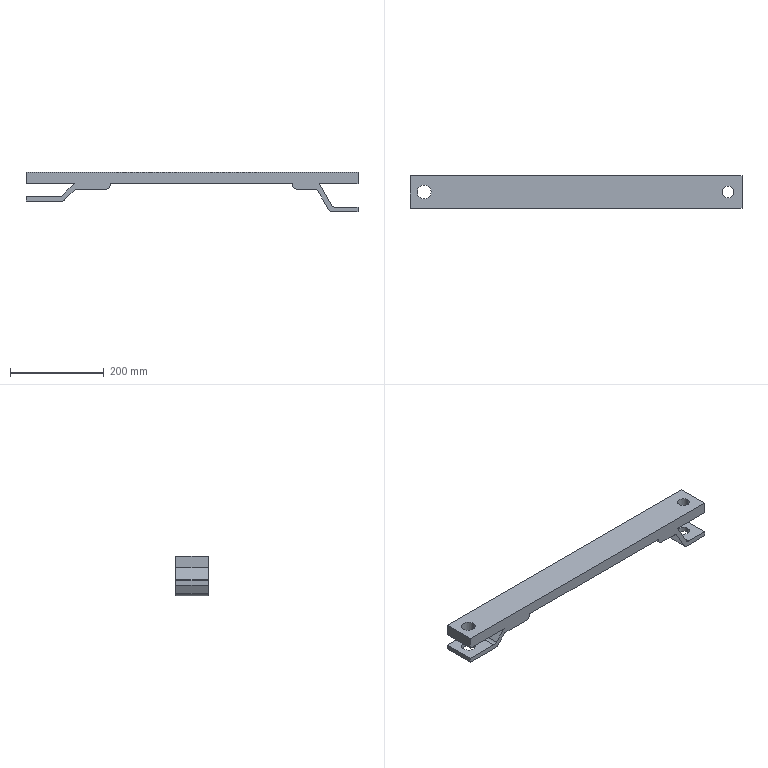Part | SolidWorks | 1 solid | 37 faces | box 710 x 70 x 85 mm | volume 1467586 mm3 | plane 22 | cylinder 15 | commonest cylinder face diameters 20 x7 25 x4 30 x4
STEP:
#1=CARTESIAN_POINT('',(692.5,35.,0.));
#2=VERTEX_POINT('',#1);
#3=CARTESIAN_POINT('',(667.5,35.,0.));
#4=VERTEX_POINT('',#3);
#5=CARTESIAN_POINT('',(680.,35.,0.));
#6=DIRECTION('',(0.,0.,-1.));
#7=DIRECTION('',(-1.,0.,0.));
#8=AXIS2_PLACEMENT_3D('',#5,#6,#7);
#9=CIRCLE('',#8,12.5);
#10=EDGE_CURVE('',#2,#4,#9,.T.);
#11=ORIENTED_EDGE('',*,*,#10,.F.);
#12=CARTESIAN_POINT('',(692.5,35.,-25.));
#13=VERTEX_POINT('',#12);
#14=CARTESIAN_POINT('',(692.5,35.,39.));
#15=DIRECTION('',(0.,0.,-1.));
#16=VECTOR('',#15,1000.);
#17=LINE('',#14,#16);
#18=EDGE_CURVE('',#2,#13,#17,.T.);
#19=ORIENTED_EDGE('',*,*,#18,.T.);
#20=CARTESIAN_POINT('',(667.5,35.,-25.));
#21=VERTEX_POINT('',#20);
#22=CARTESIAN_POINT('',(680.,35.,-25.));
#23=DIRECTION('',(0.,0.,-1.));
#24=DIRECTION('',(-1.,0.,0.));
#25=AXIS2_PLACEMENT_3D('',#22,#23,#24);
#26=CIRCLE('',#25,12.5);
#27=EDGE_CURVE('',#13,#21,#26,.T.);
#28=ORIENTED_EDGE('',*,*,#27,.T.);
#29=CARTESIAN_POINT('',(667.5,35.,39.));
#30=DIRECTION('',(0.,0.,-1.));
#31=VECTOR('',#30,1000.);
#32=LINE('',#29,#31);
#33=EDGE_CURVE('',#4,#21,#32,.T.);
#34=ORIENTED_EDGE('',*,*,#33,.F.);
#35=EDGE_LOOP('',(#11,#19,#28,#34));
#36=FACE_OUTER_BOUND('',#35,.T.);
#37=CARTESIAN_POINT('',(680.,35.,39.));
#38=DIRECTION('',(0.,0.,-1.));
#39=DIRECTION('',(-1.,0.,0.));
#40=AXIS2_PLACEMENT_3D('',#37,#38,#39);
#41=CYLINDRICAL_SURFACE('',#40,12.5);
#42=ADVANCED_FACE('',(#36),#41,.F.);
#43=CARTESIAN_POINT('',(692.5,35.,-75.));
#44=VERTEX_POINT('',#43);
#45=CARTESIAN_POINT('',(667.5,35.,-75.));
#46=VERTEX_POINT('',#45);
#47=CARTESIAN_POINT('',(680.,35.,-75.));
#48=DIRECTION('',(0.,0.,-1.));
#49=DIRECTION('',(-1.,0.,0.));
#50=AXIS2_PLACEMENT_3D('',#47,#48,#49);
#51=CIRCLE('',#50,12.5);
#52=EDGE_CURVE('',#44,#46,#51,.T.);
#53=ORIENTED_EDGE('',*,*,#52,.F.);
#54=CARTESIAN_POINT('',(692.5,35.,-85.));
#55=VERTEX_POINT('',#54);
#56=CARTESIAN_POINT('',(692.5,35.,39.));
#57=DIRECTION('',(0.,0.,-1.));
#58=VECTOR('',#57,1000.);
#59=LINE('',#56,#58);
#60=EDGE_CURVE('',#44,#55,#59,.T.);
#61=ORIENTED_EDGE('',*,*,#60,.T.);
#62=CARTESIAN_POINT('',(667.5,35.,-85.));
#63=VERTEX_POINT('',#62);
#64=CARTESIAN_POINT('',(680.,35.,-85.));
#65=DIRECTION('',(0.,0.,-1.));
#66=DIRECTION('',(-1.,0.,0.));
#67=AXIS2_PLACEMENT_3D('',#64,#65,#66);
#68=CIRCLE('',#67,12.5);
#69=EDGE_CURVE('',#55,#63,#68,.T.);
#70=ORIENTED_EDGE('',*,*,#69,.T.);
#71=CARTESIAN_POINT('',(667.5,35.,39.));
#72=DIRECTION('',(0.,0.,-1.));
#73=VECTOR('',#72,1000.);
#74=LINE('',#71,#73);
#75=EDGE_CURVE('',#46,#63,#74,.T.);
#76=ORIENTED_EDGE('',*,*,#75,.F.);
#77=EDGE_LOOP('',(#53,#61,#70,#76));
#78=FACE_OUTER_BOUND('',#77,.T.);
#79=CARTESIAN_POINT('',(680.,35.,39.));
#80=DIRECTION('',(0.,0.,-1.));
#81=DIRECTION('',(-1.,0.,0.));
#82=AXIS2_PLACEMENT_3D('',#79,#80,#81);
#83=CYLINDRICAL_SURFACE('',#82,12.5);
#84=ADVANCED_FACE('',(#78),#83,.F.);
#85=CARTESIAN_POINT('',(45.,35.,-52.));
#86=VERTEX_POINT('',#85);
#87=CARTESIAN_POINT('',(15.,35.,-52.));
#88=VERTEX_POINT('',#87);
#89=CARTESIAN_POINT('',(30.,35.,-52.));
#90=DIRECTION('',(0.,0.,-1.));
#91=DIRECTION('',(-1.,0.,0.));
#92=AXIS2_PLACEMENT_3D('',#89,#90,#91);
#93=CIRCLE('',#92,15.);
#94=EDGE_CURVE('',#86,#88,#93,.T.);
#95=ORIENTED_EDGE('',*,*,#94,.F.);
#96=CARTESIAN_POINT('',(45.,35.,-62.));
#97=VERTEX_POINT('',#96);
#98=CARTESIAN_POINT('',(45.,35.,39.));
#99=DIRECTION('',(0.,0.,-1.));
#100=VECTOR('',#99,1000.);
#101=LINE('',#98,#100);
#102=EDGE_CURVE('',#86,#97,#101,.T.);
#103=ORIENTED_EDGE('',*,*,#102,.T.);
#104=CARTESIAN_POINT('',(15.,35.,-62.));
#105=VERTEX_POINT('',#104);
#106=CARTESIAN_POINT('',(30.,35.,-62.));
#107=DIRECTION('',(0.,0.,-1.));
#108=DIRECTION('',(-1.,0.,0.));
#109=AXIS2_PLACEMENT_3D('',#106,#107,#108);
#110=CIRCLE('',#109,15.);
#111=EDGE_CURVE('',#97,#105,#110,.T.);
#112=ORIENTED_EDGE('',*,*,#111,.T.);
#113=CARTESIAN_POINT('',(15.,35.,39.));
#114=DIRECTION('',(0.,0.,-1.));
#115=VECTOR('',#114,1000.);
#116=LINE('',#113,#115);
#117=EDGE_CURVE('',#88,#105,#116,.T.);
#118=ORIENTED_EDGE('',*,*,#117,.F.);
#119=EDGE_LOOP('',(#95,#103,#112,#118));
#120=FACE_OUTER_BOUND('',#119,.T.);
#121=CARTESIAN_POINT('',(30.,35.,39.));
#122=DIRECTION('',(0.,0.,-1.));
#123=DIRECTION('',(-1.,0.,0.));
#124=AXIS2_PLACEMENT_3D('',#121,#122,#123);
#125=CYLINDRICAL_SURFACE('',#124,15.);
#126=ADVANCED_FACE('',(#120),#125,.F.);
#127=CARTESIAN_POINT('',(45.,35.,0.));
#128=VERTEX_POINT('',#127);
#129=CARTESIAN_POINT('',(15.,35.,0.));
#130=VERTEX_POINT('',#129);
#131=CARTESIAN_POINT('',(30.,35.,0.));
#132=DIRECTION('',(0.,0.,-1.));
#133=DIRECTION('',(-1.,0.,0.));
#134=AXIS2_PLACEMENT_3D('',#131,#132,#133);
#135=CIRCLE('',#134,15.);
#136=EDGE_CURVE('',#128,#130,#135,.T.);
#137=ORIENTED_EDGE('',*,*,#136,.F.);
#138=CARTESIAN_POINT('',(45.,35.,-25.));
#139=VERTEX_POINT('',#138);
#140=CARTESIAN_POINT('',(45.,35.,39.));
#141=DIRECTION('',(0.,0.,-1.));
#142=VECTOR('',#141,1000.);
#143=LINE('',#140,#142);
#144=EDGE_CURVE('',#128,#139,#143,.T.);
#145=ORIENTED_EDGE('',*,*,#144,.T.);
#146=CARTESIAN_POINT('',(15.,35.,-25.));
#147=VERTEX_POINT('',#146);
#148=CARTESIAN_POINT('',(30.,35.,-25.));
#149=DIRECTION('',(0.,0.,-1.));
#150=DIRECTION('',(-1.,0.,0.));
#151=AXIS2_PLACEMENT_3D('',#148,#149,#150);
#152=CIRCLE('',#151,15.);
#153=EDGE_CURVE('',#139,#147,#152,.T.);
#154=ORIENTED_EDGE('',*,*,#153,.T.);
#155=CARTESIAN_POINT('',(15.,35.,39.));
#156=DIRECTION('',(0.,0.,-1.));
#157=VECTOR('',#156,1000.);
#158=LINE('',#155,#157);
#159=EDGE_CURVE('',#130,#147,#158,.T.);
#160=ORIENTED_EDGE('',*,*,#159,.F.);
#161=EDGE_LOOP('',(#137,#145,#154,#160));
#162=FACE_OUTER_BOUND('',#161,.T.);
#163=CARTESIAN_POINT('',(30.,35.,39.));
#164=DIRECTION('',(0.,0.,-1.));
#165=DIRECTION('',(-1.,0.,0.));
#166=AXIS2_PLACEMENT_3D('',#163,#164,#165);
#167=CYLINDRICAL_SURFACE('',#166,15.);
#168=ADVANCED_FACE('',(#162),#167,.F.);
#169=CARTESIAN_POINT('',(680.,35.,0.));
#170=DIRECTION('',(0.,0.,-1.));
#171=DIRECTION('',(-1.,0.,0.));
#172=AXIS2_PLACEMENT_3D('',#169,#170,#171);
#173=CIRCLE('',#172,12.5);
#174=EDGE_CURVE('',#4,#2,#173,.T.);
#175=ORIENTED_EDGE('',*,*,#174,.T.);
#176=ORIENTED_EDGE('',*,*,#10,.T.);
#177=EDGE_LOOP('',(#175,#176));
#178=FACE_BOUND('',#177,.T.);
#179=CARTESIAN_POINT('',(30.,35.,0.));
#180=DIRECTION('',(0.,0.,-1.));
#181=DIRECTION('',(-1.,0.,0.));
#182=AXIS2_PLACEMENT_3D('',#179,#180,#181);
#183=CIRCLE('',#182,15.);
#184=EDGE_CURVE('',#130,#128,#183,.T.);
#185=ORIENTED_EDGE('',*,*,#184,.T.);
#186=ORIENTED_EDGE('',*,*,#136,.T.);
#187=EDGE_LOOP('',(#185,#186));
#188=FACE_BOUND('',#187,.T.);
#189=CARTESIAN_POINT('',(0.,0.,0.));
#190=VERTEX_POINT('',#189);
#191=CARTESIAN_POINT('',(710.,0.,0.));
#192=VERTEX_POINT('',#191);
#193=CARTESIAN_POINT('',(0.,0.,0.));
#194=DIRECTION('',(1.,0.,0.));
#195=VECTOR('',#194,1000.);
#196=LINE('',#193,#195);
#197=EDGE_CURVE('',#190,#192,#196,.T.);
#198=ORIENTED_EDGE('',*,*,#197,.T.);
#199=CARTESIAN_POINT('',(710.,70.,0.));
#200=VERTEX_POINT('',#199);
#201=CARTESIAN_POINT('',(710.,70.,0.));
#202=DIRECTION('',(0.,-1.,0.));
#203=VECTOR('',#202,1000.);
#204=LINE('',#201,#203);
#205=EDGE_CURVE('',#200,#192,#204,.T.);
#206=ORIENTED_EDGE('',*,*,#205,.F.);
#207=CARTESIAN_POINT('',(0.,70.,0.));
#208=VERTEX_POINT('',#207);
#209=CARTESIAN_POINT('',(0.,70.,0.));
#210=DIRECTION('',(1.,0.,0.));
#211=VECTOR('',#210,1000.);
#212=LINE('',#209,#211);
#213=EDGE_CURVE('',#208,#200,#212,.T.);
#214=ORIENTED_EDGE('',*,*,#213,.F.);
#215=CARTESIAN_POINT('',(0.,70.,0.));
#216=DIRECTION('',(0.,-1.,0.));
#217=VECTOR('',#216,1000.);
#218=LINE('',#215,#217);
#219=EDGE_CURVE('',#208,#190,#218,.T.);
#220=ORIENTED_EDGE('',*,*,#219,.T.);
#221=EDGE_LOOP('',(#198,#206,#214,#220));
#222=FACE_OUTER_BOUND('',#221,.T.);
#223=CARTESIAN_POINT('',(0.,70.,0.));
#224=DIRECTION('',(0.,0.,-1.));
#225=DIRECTION('',(-1.,0.,0.));
#226=AXIS2_PLACEMENT_3D('',#223,#224,#225);
#227=PLANE('',#226);
#228=ADVANCED_FACE('',(#178,#188,#222),#227,.F.);
#229=CARTESIAN_POINT('',(710.,0.,-25.));
#230=VERTEX_POINT('',#229);
#231=CARTESIAN_POINT('',(710.,0.,0.));
#232=DIRECTION('',(0.,0.,-1.));
#233=VECTOR('',#232,1000.);
#234=LINE('',#231,#233);
#235=EDGE_CURVE('',#192,#230,#234,.T.);
#236=ORIENTED_EDGE('',*,*,#235,.T.);
#237=CARTESIAN_POINT('',(710.,70.,-25.));
#238=VERTEX_POINT('',#237);
#239=CARTESIAN_POINT('',(710.,70.,-25.));
#240=DIRECTION('',(0.,-1.,0.));
#241=VECTOR('',#240,1000.);
#242=LINE('',#239,#241);
#243=EDGE_CURVE('',#238,#230,#242,.T.);
#244=ORIENTED_EDGE('',*,*,#243,.F.);
#245=CARTESIAN_POINT('',(710.,70.,0.));
#246=DIRECTION('',(0.,0.,-1.));
#247=VECTOR('',#246,1000.);
#248=LINE('',#245,#247);
#249=EDGE_CURVE('',#200,#238,#248,.T.);
#250=ORIENTED_EDGE('',*,*,#249,.F.);
#251=ORIENTED_EDGE('',*,*,#205,.T.);
#252=EDGE_LOOP('',(#236,#244,#250,#251));
#253=FACE_OUTER_BOUND('',#252,.T.);
#254=CARTESIAN_POINT('',(710.,70.,0.));
#255=DIRECTION('',(-1.,0.,0.));
#256=DIRECTION('',(0.,0.,1.));
#257=AXIS2_PLACEMENT_3D('',#254,#255,#256);
#258=PLANE('',#257);
#259=ADVANCED_FACE('',(#253),#258,.F.);
#260=CARTESIAN_POINT('',(680.,35.,-25.));
#261=DIRECTION('',(0.,0.,-1.));
#262=DIRECTION('',(-1.,0.,0.));
#263=AXIS2_PLACEMENT_3D('',#260,#261,#262);
#264=CIRCLE('',#263,12.5);
#265=EDGE_CURVE('',#21,#13,#264,.T.);
#266=ORIENTED_EDGE('',*,*,#265,.F.);
#267=ORIENTED_EDGE('',*,*,#27,.F.);
#268=EDGE_LOOP('',(#266,#267));
#269=FACE_BOUND('',#268,.T.);
#270=CARTESIAN_POINT('',(626.906,0.,-25.));
#271=VERTEX_POINT('',#270);
#272=CARTESIAN_POINT('',(0.,0.,-25.));
#273=DIRECTION('',(1.,0.,0.));
#274=VECTOR('',#273,1000.);
#275=LINE('',#272,#274);
#276=EDGE_CURVE('',#271,#230,#275,.T.);
#277=ORIENTED_EDGE('',*,*,#276,.F.);
#278=CARTESIAN_POINT('',(626.906,70.,-25.));
#279=VERTEX_POINT('',#278);
#280=CARTESIAN_POINT('',(626.906,70.,-25.));
#281=DIRECTION('',(0.,-1.,0.));
#282=VECTOR('',#281,1000.);
#283=LINE('',#280,#282);
#284=EDGE_CURVE('',#279,#271,#283,.T.);
#285=ORIENTED_EDGE('',*,*,#284,.F.);
#286=CARTESIAN_POINT('',(0.,70.,-25.));
#287=DIRECTION('',(1.,0.,0.));
#288=VECTOR('',#287,1000.);
#289=LINE('',#286,#288);
#290=EDGE_CURVE('',#279,#238,#289,.T.);
#291=ORIENTED_EDGE('',*,*,#290,.T.);
#292=ORIENTED_EDGE('',*,*,#243,.T.);
#293=EDGE_LOOP('',(#277,#285,#291,#292));
#294=FACE_OUTER_BOUND('',#293,.T.);
#295=CARTESIAN_POINT('',(0.,70.,-25.));
#296=DIRECTION('',(0.,0.,-1.));
#297=DIRECTION('',(-1.,0.,0.));
#298=AXIS2_PLACEMENT_3D('',#295,#296,#297);
#299=PLANE('',#298);
#300=ADVANCED_FACE('',(#269,#294),#299,.T.);
#301=CARTESIAN_POINT('',(652.887,0.,-70.));
#302=VERTEX_POINT('',#301);
#303=CARTESIAN_POINT('',(459.354,0.,265.208));
#304=DIRECTION('',(0.5,0.,-0.866));
#305=VECTOR('',#304,1000.);
#306=LINE('',#303,#305);
#307=EDGE_CURVE('',#271,#302,#306,.T.);
#308=ORIENTED_EDGE('',*,*,#307,.T.);
#309=CARTESIAN_POINT('',(652.887,70.,-70.));
#310=VERTEX_POINT('',#309);
#311=CARTESIAN_POINT('',(652.887,70.,-70.));
#312=DIRECTION('',(0.,1.,0.));
#313=VECTOR('',#312,1000.);
#314=LINE('',#311,#313);
#315=EDGE_CURVE('',#302,#310,#314,.T.);
#316=ORIENTED_EDGE('',*,*,#315,.T.);
#317=CARTESIAN_POINT('',(459.354,70.,265.208));
#318=DIRECTION('',(0.5,0.,-0.866));
#319=VECTOR('',#318,1000.);
#320=LINE('',#317,#319);
#321=EDGE_CURVE('',#279,#310,#320,.T.);
#322=ORIENTED_EDGE('',*,*,#321,.F.);
#323=ORIENTED_EDGE('',*,*,#284,.T.);
#324=EDGE_LOOP('',(#308,#316,#322,#323));
#325=FACE_OUTER_BOUND('',#324,.T.);
#326=CARTESIAN_POINT('',(459.354,70.,265.208));
#327=DIRECTION('',(-0.866,0.,-0.5));
#328=DIRECTION('',(-0.5,0.,0.866));
#329=AXIS2_PLACEMENT_3D('',#326,#327,#328);
#330=PLANE('',#329);
#331=ADVANCED_FACE('',(#325),#330,.F.);
#332=CARTESIAN_POINT('',(680.,35.,-75.));
#333=DIRECTION('',(0.,0.,-1.));
#334=DIRECTION('',(-1.,0.,0.));
#335=AXIS2_PLACEMENT_3D('',#332,#333,#334);
#336=CIRCLE('',#335,12.5);
#337=EDGE_CURVE('',#46,#44,#336,.T.);
#338=ORIENTED_EDGE('',*,*,#337,.T.);
#339=ORIENTED_EDGE('',*,*,#52,.T.);
#340=EDGE_LOOP('',(#338,#339));
#341=FACE_BOUND('',#340,.T.);
#342=CARTESIAN_POINT('',(661.547,70.,-75.));
#343=VERTEX_POINT('',#342);
#344=CARTESIAN_POINT('',(710.,70.,-75.));
#345=VERTEX_POINT('',#344);
#346=CARTESIAN_POINT('',(0.,70.,-75.));
#347=DIRECTION('',(1.,0.,0.));
#348=VECTOR('',#347,1000.);
#349=LINE('',#346,#348);
#350=EDGE_CURVE('',#343,#345,#349,.T.);
#351=ORIENTED_EDGE('',*,*,#350,.F.);
#352=CARTESIAN_POINT('',(661.547,0.,-75.));
#353=VERTEX_POINT('',#352);
#354=CARTESIAN_POINT('',(661.547,0.,-75.));
#355=DIRECTION('',(0.,-1.,0.));
#356=VECTOR('',#355,1000.);
#357=LINE('',#354,#356);
#358=EDGE_CURVE('',#343,#353,#357,.T.);
#359=ORIENTED_EDGE('',*,*,#358,.T.);
#360=CARTESIAN_POINT('',(710.,0.,-75.));
#361=VERTEX_POINT('',#360);
#362=CARTESIAN_POINT('',(0.,0.,-75.));
#363=DIRECTION('',(1.,0.,0.));
#364=VECTOR('',#363,1000.);
#365=LINE('',#362,#364);
#366=EDGE_CURVE('',#353,#361,#365,.T.);
#367=ORIENTED_EDGE('',*,*,#366,.T.);
#368=CARTESIAN_POINT('',(710.,70.,-75.));
#369=DIRECTION('',(0.,-1.,0.));
#370=VECTOR('',#369,1000.);
#371=LINE('',#368,#370);
#372=EDGE_CURVE('',#345,#361,#371,.T.);
#373=ORIENTED_EDGE('',*,*,#372,.F.);
#374=EDGE_LOOP('',(#351,#359,#367,#373));
#375=FACE_OUTER_BOUND('',#374,.T.);
#376=CARTESIAN_POINT('',(0.,70.,-75.));
#377=DIRECTION('',(0.,0.,-1.));
#378=DIRECTION('',(-1.,0.,0.));
#379=AXIS2_PLACEMENT_3D('',#376,#377,#378);
#380=PLANE('',#379);
#381=ADVANCED_FACE('',(#341,#375),#380,.F.);
#382=CARTESIAN_POINT('',(710.,0.,-85.));
#383=VERTEX_POINT('',#382);
#384=CARTESIAN_POINT('',(710.,0.,0.));
#385=DIRECTION('',(0.,0.,1.));
#386=VECTOR('',#385,1000.);
#387=LINE('',#384,#386);
#388=EDGE_CURVE('',#383,#361,#387,.T.);
#389=ORIENTED_EDGE('',*,*,#388,.F.);
#390=CARTESIAN_POINT('',(710.,70.,-85.));
#391=VERTEX_POINT('',#390);
#392=CARTESIAN_POINT('',(710.,70.,-85.));
#393=DIRECTION('',(0.,-1.,0.));
#394=VECTOR('',#393,1000.);
#395=LINE('',#392,#394);
#396=EDGE_CURVE('',#391,#383,#395,.T.);
#397=ORIENTED_EDGE('',*,*,#396,.F.);
#398=CARTESIAN_POINT('',(710.,70.,0.));
#399=DIRECTION('',(0.,0.,1.));
#400=VECTOR('',#399,1000.);
#401=LINE('',#398,#400);
#402=EDGE_CURVE('',#391,#345,#401,.T.);
#403=ORIENTED_EDGE('',*,*,#402,.T.);
#404=ORIENTED_EDGE('',*,*,#372,.T.);
#405=EDGE_LOOP('',(#389,#397,#403,#404));
#406=FACE_OUTER_BOUND('',#405,.T.);
#407=CARTESIAN_POINT('',(710.,70.,0.));
#408=DIRECTION('',(1.,0.,0.));
#409=DIRECTION('',(0.,0.,-1.));
#410=AXIS2_PLACEMENT_3D('',#407,#408,#409);
#411=PLANE('',#410);
#412=ADVANCED_FACE('',(#406),#411,.T.);
#413=CARTESIAN_POINT('',(680.,35.,-85.));
#414=DIRECTION('',(0.,0.,-1.));
#415=DIRECTION('',(-1.,0.,0.));
#416=AXIS2_PLACEMENT_3D('',#413,#414,#415);
#417=CIRCLE('',#416,12.5);
#418=EDGE_CURVE('',#63,#55,#417,.T.);
#419=ORIENTED_EDGE('',*,*,#418,.F.);
#420=ORIENTED_EDGE('',*,*,#69,.F.);
#421=EDGE_LOOP('',(#419,#420));
#422=FACE_BOUND('',#421,.T.);
#423=CARTESIAN_POINT('',(655.774,0.,-85.));
#424=VERTEX_POINT('',#423);
#425=CARTESIAN_POINT('',(0.,0.,-85.));
#426=DIRECTION('',(1.,0.,0.));
#427=VECTOR('',#426,1000.);
#428=LINE('',#425,#427);
#429=EDGE_CURVE('',#424,#383,#428,.T.);
#430=ORIENTED_EDGE('',*,*,#429,.F.);
#431=CARTESIAN_POINT('',(655.774,70.,-85.));
#432=VERTEX_POINT('',#431);
#433=CARTESIAN_POINT('',(655.774,70.,-85.));
#434=DIRECTION('',(0.,1.,0.));
#435=VECTOR('',#434,1000.);
#436=LINE('',#433,#435);
#437=EDGE_CURVE('',#424,#432,#436,.T.);
#438=ORIENTED_EDGE('',*,*,#437,.T.);
#439=CARTESIAN_POINT('',(0.,70.,-85.));
#440=DIRECTION('',(1.,0.,0.));
#441=VECTOR('',#440,1000.);
#442=LINE('',#439,#441);
#443=EDGE_CURVE('',#432,#391,#442,.T.);
#444=ORIENTED_EDGE('',*,*,#443,.T.);
#445=ORIENTED_EDGE('',*,*,#396,.T.);
#446=EDGE_LOOP('',(#430,#438,#444,#445));
#447=FACE_OUTER_BOUND('',#446,.T.);
#448=CARTESIAN_POINT('',(0.,70.,-85.));
#449=DIRECTION('',(0.,0.,-1.));
#450=DIRECTION('',(-1.,0.,0.));
#451=AXIS2_PLACEMENT_3D('',#448,#449,#450);
#452=PLANE('',#451);
#453=ADVANCED_FACE('',(#422,#447),#452,.T.);
#454=CARTESIAN_POINT('',(625.174,0.,-42.));
#455=VERTEX_POINT('',#454);
#456=CARTESIAN_POINT('',(647.113,0.,-80.));
#457=VERTEX_POINT('',#456);
#458=CARTESIAN_POINT('',(450.694,0.,260.208));
#459=DIRECTION('',(0.5,0.,-0.866));
#460=VECTOR('',#459,1000.);
#461=LINE('',#458,#460);
#462=EDGE_CURVE('',#455,#457,#461,.T.);
#463=ORIENTED_EDGE('',*,*,#462,.F.);
#464=CARTESIAN_POINT('',(625.174,70.,-42.));
#465=VERTEX_POINT('',#464);
#466=CARTESIAN_POINT('',(625.174,70.,-42.));
#467=DIRECTION('',(0.,1.,0.));
#468=VECTOR('',#467,1000.);
#469=LINE('',#466,#468);
#470=EDGE_CURVE('',#455,#465,#469,.T.);
#471=ORIENTED_EDGE('',*,*,#470,.T.);
#472=CARTESIAN_POINT('',(647.113,70.,-80.));
#473=VERTEX_POINT('',#472);
#474=CARTESIAN_POINT('',(450.694,70.,260.208));
#475=DIRECTION('',(0.5,0.,-0.866));
#476=VECTOR('',#475,1000.);
#477=LINE('',#474,#476);
#478=EDGE_CURVE('',#465,#473,#477,.T.);
#479=ORIENTED_EDGE('',*,*,#478,.T.);
#480=CARTESIAN_POINT('',(647.113,70.,-80.));
#481=DIRECTION('',(0.,-1.,0.));
#482=VECTOR('',#481,1000.);
#483=LINE('',#480,#482);
#484=EDGE_CURVE('',#473,#457,#483,.T.);
#485=ORIENTED_EDGE('',*,*,#484,.T.);
#486=EDGE_LOOP('',(#463,#471,#479,#485));
#487=FACE_OUTER_BOUND('',#486,.T.);
#488=CARTESIAN_POINT('',(450.694,70.,260.208));
#489=DIRECTION('',(-0.866,0.,-0.5));
#490=DIRECTION('',(-0.5,0.,0.866));
#491=AXIS2_PLACEMENT_3D('',#488,#489,#490);
#492=PLANE('',#491);
#493=ADVANCED_FACE('',(#487),#492,.T.);
#494=CARTESIAN_POINT('',(580.,0.,-37.));
#495=VERTEX_POINT('',#494);
#496=CARTESIAN_POINT('',(616.514,0.,-37.));
#497=VERTEX_POINT('',#496);
#498=CARTESIAN_POINT('',(0.,0.,-37.));
#499=DIRECTION('',(1.,0.,0.));
#500=VECTOR('',#499,1000.);
#501=LINE('',#498,#500);
#502=EDGE_CURVE('',#495,#497,#501,.T.);
#503=ORIENTED_EDGE('',*,*,#502,.F.);
#504=CARTESIAN_POINT('',(580.,70.,-37.));
#505=VERTEX_POINT('',#504);
#506=CARTESIAN_POINT('',(580.,70.,-37.));
#507=DIRECTION('',(0.,1.,0.));
#508=VECTOR('',#507,1000.);
#509=LINE('',#506,#508);
#510=EDGE_CURVE('',#495,#505,#509,.T.);
#511=ORIENTED_EDGE('',*,*,#510,.T.);
#512=CARTESIAN_POINT('',(616.514,70.,-37.));
#513=VERTEX_POINT('',#512);
#514=CARTESIAN_POINT('',(0.,70.,-37.));
#515=DIRECTION('',(1.,0.,0.));
#516=VECTOR('',#515,1000.);
#517=LINE('',#514,#516);
#518=EDGE_CURVE('',#505,#513,#517,.T.);
#519=ORIENTED_EDGE('',*,*,#518,.T.);
#520=CARTESIAN_POINT('',(616.514,0.,-37.));
#521=DIRECTION('',(0.,-1.,0.));
#522=VECTOR('',#521,1000.);
#523=LINE('',#520,#522);
#524=EDGE_CURVE('',#513,#497,#523,.T.);
#525=ORIENTED_EDGE('',*,*,#524,.T.);
#526=EDGE_LOOP('',(#503,#511,#519,#525));
#527=FACE_OUTER_BOUND('',#526,.T.);
#528=CARTESIAN_POINT('',(0.,70.,-37.));
#529=DIRECTION('',(0.,0.,-1.));
#530=DIRECTION('',(-1.,0.,0.));
#531=AXIS2_PLACEMENT_3D('',#528,#529,#530);
#532=PLANE('',#531);
#533=ADVANCED_FACE('',(#527),#532,.T.);
#534=CARTESIAN_POINT('',(570.,70.,-25.));
#535=VERTEX_POINT('',#534);
#536=CARTESIAN_POINT('',(570.,70.,-27.));
#537=VERTEX_POINT('',#536);
#538=CARTESIAN_POINT('',(570.,70.,0.));
#539=DIRECTION('',(0.,0.,-1.));
#540=VECTOR('',#539,1000.);
#541=LINE('',#538,#540);
#542=EDGE_CURVE('',#535,#537,#541,.T.);
#543=ORIENTED_EDGE('',*,*,#542,.T.);
#544=CARTESIAN_POINT('',(570.,0.,-27.));
#545=VERTEX_POINT('',#544);
#546=CARTESIAN_POINT('',(570.,70.,-27.));
#547=DIRECTION('',(0.,-1.,0.));
#548=VECTOR('',#547,1000.);
#549=LINE('',#546,#548);
#550=EDGE_CURVE('',#537,#545,#549,.T.);
#551=ORIENTED_EDGE('',*,*,#550,.T.);
#552=CARTESIAN_POINT('',(570.,0.,-25.));
#553=VERTEX_POINT('',#552);
#554=CARTESIAN_POINT('',(570.,0.,0.));
#555=DIRECTION('',(0.,0.,-1.));
#556=VECTOR('',#555,1000.);
#557=LINE('',#554,#556);
#558=EDGE_CURVE('',#553,#545,#557,.T.);
#559=ORIENTED_EDGE('',*,*,#558,.F.);
#560=CARTESIAN_POINT('',(570.,70.,-25.));
#561=DIRECTION('',(0.,-1.,0.));
#562=VECTOR('',#561,1000.);
#563=LINE('',#560,#562);
#564=EDGE_CURVE('',#535,#553,#563,.T.);
#565=ORIENTED_EDGE('',*,*,#564,.F.);
#566=EDGE_LOOP('',(#543,#551,#559,#565));
#567=FACE_OUTER_BOUND('',#566,.T.);
#568=CARTESIAN_POINT('',(570.,70.,0.));
#569=DIRECTION('',(-1.,0.,0.));
#570=DIRECTION('',(0.,0.,1.));
#571=AXIS2_PLACEMENT_3D('',#568,#569,#570);
#572=PLANE('',#571);
#573=ADVANCED_FACE('',(#567),#572,.T.);
#574=CARTESIAN_POINT('',(180.,0.,-25.));
#575=VERTEX_POINT('',#574);
#576=CARTESIAN_POINT('',(0.,0.,-25.));
#577=DIRECTION('',(1.,0.,0.));
#578=VECTOR('',#577,1000.);
#579=LINE('',#576,#578);
#580=EDGE_CURVE('',#575,#553,#579,.T.);
#581=ORIENTED_EDGE('',*,*,#580,.F.);
#582=CARTESIAN_POINT('',(180.,70.,-25.));
#583=VERTEX_POINT('',#582);
#584=CARTESIAN_POINT('',(180.,70.,-25.));
#585=DIRECTION('',(0.,-1.,0.));
#586=VECTOR('',#585,1000.);
#587=LINE('',#584,#586);
#588=EDGE_CURVE('',#583,#575,#587,.T.);
#589=ORIENTED_EDGE('',*,*,#588,.F.);
#590=CARTESIAN_POINT('',(0.,70.,-25.));
#591=DIRECTION('',(1.,0.,0.));
#592=VECTOR('',#591,1000.);
#593=LINE('',#590,#592);
#594=EDGE_CURVE('',#583,#535,#593,.T.);
#595=ORIENTED_EDGE('',*,*,#594,.T.);
#596=ORIENTED_EDGE('',*,*,#564,.T.);
#597=EDGE_LOOP('',(#581,#589,#595,#596));
#598=FACE_OUTER_BOUND('',#597,.T.);
#599=CARTESIAN_POINT('',(0.,70.,-25.));
#600=DIRECTION('',(0.,0.,-1.));
#601=DIRECTION('',(-1.,0.,0.));
#602=AXIS2_PLACEMENT_3D('',#599,#600,#601);
#603=PLANE('',#602);
#604=ADVANCED_FACE('',(#598),#603,.T.);
#605=CARTESIAN_POINT('',(180.,0.,-27.));
#606=VERTEX_POINT('',#605);
#607=CARTESIAN_POINT('',(180.,0.,0.));
#608=DIRECTION('',(0.,0.,1.));
#609=VECTOR('',#608,1000.);
#610=LINE('',#607,#609);
#611=EDGE_CURVE('',#606,#575,#610,.T.);
#612=ORIENTED_EDGE('',*,*,#611,.F.);
#613=CARTESIAN_POINT('',(180.,70.,-27.));
#614=VERTEX_POINT('',#613);
#615=CARTESIAN_POINT('',(180.,70.,-27.));
#616=DIRECTION('',(0.,1.,0.));
#617=VECTOR('',#616,1000.);
#618=LINE('',#615,#617);
#619=EDGE_CURVE('',#606,#614,#618,.T.);
#620=ORIENTED_EDGE('',*,*,#619,.T.);
#621=CARTESIAN_POINT('',(180.,70.,0.));
#622=DIRECTION('',(0.,0.,1.));
#623=VECTOR('',#622,1000.);
#624=LINE('',#621,#623);
#625=EDGE_CURVE('',#614,#583,#624,.T.);
#626=ORIENTED_EDGE('',*,*,#625,.T.);
#627=ORIENTED_EDGE('',*,*,#588,.T.);
#628=EDGE_LOOP('',(#612,#620,#626,#627));
#629=FACE_OUTER_BOUND('',#628,.T.);
#630=CARTESIAN_POINT('',(180.,70.,0.));
#631=DIRECTION('',(1.,0.,0.));
#632=DIRECTION('',(0.,0.,-1.));
#633=AXIS2_PLACEMENT_3D('',#630,#631,#632);
#634=PLANE('',#633);
#635=ADVANCED_FACE('',(#629),#634,.T.);
#636=CARTESIAN_POINT('',(105.,70.,-37.));
#637=VERTEX_POINT('',#636);
#638=CARTESIAN_POINT('',(170.,70.,-37.));
#639=VERTEX_POINT('',#638);
#640=CARTESIAN_POINT('',(0.,70.,-37.));
#641=DIRECTION('',(1.,0.,0.));
#642=VECTOR('',#641,1000.);
#643=LINE('',#640,#642);
#644=EDGE_CURVE('',#637,#639,#643,.T.);
#645=ORIENTED_EDGE('',*,*,#644,.T.);
#646=CARTESIAN_POINT('',(170.,0.,-37.));
#647=VERTEX_POINT('',#646);
#648=CARTESIAN_POINT('',(170.,70.,-37.));
#649=DIRECTION('',(0.,-1.,0.));
#650=VECTOR('',#649,1000.);
#651=LINE('',#648,#650);
#652=EDGE_CURVE('',#639,#647,#651,.T.);
#653=ORIENTED_EDGE('',*,*,#652,.T.);
#654=CARTESIAN_POINT('',(105.,0.,-37.));
#655=VERTEX_POINT('',#654);
#656=CARTESIAN_POINT('',(0.,0.,-37.));
#657=DIRECTION('',(1.,0.,0.));
#658=VECTOR('',#657,1000.);
#659=LINE('',#656,#658);
#660=EDGE_CURVE('',#655,#647,#659,.T.);
#661=ORIENTED_EDGE('',*,*,#660,.F.);
#662=CARTESIAN_POINT('',(105.,70.,-37.));
#663=DIRECTION('',(0.,-1.,0.));
#664=VECTOR('',#663,1000.);
#665=LINE('',#662,#664);
#666=EDGE_CURVE('',#637,#655,#665,.T.);
#667=ORIENTED_EDGE('',*,*,#666,.F.);
#668=EDGE_LOOP('',(#645,#653,#661,#667));
#669=FACE_OUTER_BOUND('',#668,.T.);
#670=CARTESIAN_POINT('',(0.,70.,-37.));
#671=DIRECTION('',(0.,0.,-1.));
#672=DIRECTION('',(-1.,0.,0.));
#673=AXIS2_PLACEMENT_3D('',#670,#671,#672);
#674=PLANE('',#673);
#675=ADVANCED_FACE('',(#669),#674,.T.);
#676=CARTESIAN_POINT('',(82.929,0.,-59.071));
#677=VERTEX_POINT('',#676);
#678=CARTESIAN_POINT('',(71.,0.,-71.));
#679=DIRECTION('',(0.7071,0.,0.7071));
#680=VECTOR('',#679,1000.);
#681=LINE('',#678,#680);
#682=EDGE_CURVE('',#677,#655,#681,.T.);
#683=ORIENTED_EDGE('',*,*,#682,.F.);
#684=CARTESIAN_POINT('',(82.929,70.,-59.071));
#685=VERTEX_POINT('',#684);
#686=CARTESIAN_POINT('',(82.929,70.,-59.071));
#687=DIRECTION('',(0.,1.,0.));
#688=VECTOR('',#687,1000.);
#689=LINE('',#686,#688);
#690=EDGE_CURVE('',#677,#685,#689,.T.);
#691=ORIENTED_EDGE('',*,*,#690,.T.);
#692=CARTESIAN_POINT('',(71.,70.,-71.));
#693=DIRECTION('',(0.7071,0.,0.7071));
#694=VECTOR('',#693,1000.);
#695=LINE('',#692,#694);
#696=EDGE_CURVE('',#685,#637,#695,.T.);
#697=ORIENTED_EDGE('',*,*,#696,.T.);
#698=ORIENTED_EDGE('',*,*,#666,.T.);
#699=EDGE_LOOP('',(#683,#691,#697,#698));
#700=FACE_OUTER_BOUND('',#699,.T.);
#701=CARTESIAN_POINT('',(71.,70.,-71.));
#702=DIRECTION('',(0.7071,0.,-0.7071));
#703=DIRECTION('',(-0.7071,0.,-0.7071));
#704=AXIS2_PLACEMENT_3D('',#701,#702,#703);
#705=PLANE('',#704);
#706=ADVANCED_FACE('',(#700),#705,.T.);
#707=CARTESIAN_POINT('',(30.,35.,-62.));
#708=DIRECTION('',(0.,0.,-1.));
#709=DIRECTION('',(-1.,0.,0.));
#710=AXIS2_PLACEMENT_3D('',#707,#708,#709);
#711=CIRCLE('',#710,15.);
#712=EDGE_CURVE('',#105,#97,#711,.T.);
#713=ORIENTED_EDGE('',*,*,#712,.F.);
#714=ORIENTED_EDGE('',*,*,#111,.F.);
#715=EDGE_LOOP('',(#713,#714));
#716=FACE_BOUND('',#715,.T.);
#717=CARTESIAN_POINT('',(0.,70.,-62.));
#718=VERTEX_POINT('',#717);
#719=CARTESIAN_POINT('',(75.858,70.,-62.));
#720=VERTEX_POINT('',#719);
#721=CARTESIAN_POINT('',(0.,70.,-62.));
#722=DIRECTION('',(1.,0.,0.));
#723=VECTOR('',#722,1000.);
#724=LINE('',#721,#723);
#725=EDGE_CURVE('',#718,#720,#724,.T.);
#726=ORIENTED_EDGE('',*,*,#725,.T.);
#727=CARTESIAN_POINT('',(75.858,0.,-62.));
#728=VERTEX_POINT('',#727);
#729=CARTESIAN_POINT('',(75.858,70.,-62.));
#730=DIRECTION('',(0.,-1.,0.));
#731=VECTOR('',#730,1000.);
#732=LINE('',#729,#731);
#733=EDGE_CURVE('',#720,#728,#732,.T.);
#734=ORIENTED_EDGE('',*,*,#733,.T.);
#735=CARTESIAN_POINT('',(0.,0.,-62.));
#736=VERTEX_POINT('',#735);
#737=CARTESIAN_POINT('',(0.,0.,-62.));
#738=DIRECTION('',(1.,0.,0.));
#739=VECTOR('',#738,1000.);
#740=LINE('',#737,#739);
#741=EDGE_CURVE('',#736,#728,#740,.T.);
#742=ORIENTED_EDGE('',*,*,#741,.F.);
#743=CARTESIAN_POINT('',(0.,70.,-62.));
#744=DIRECTION('',(0.,-1.,0.));
#745=VECTOR('',#744,1000.);
#746=LINE('',#743,#745);
#747=EDGE_CURVE('',#718,#736,#746,.T.);
#748=ORIENTED_EDGE('',*,*,#747,.F.);
#749=EDGE_LOOP('',(#726,#734,#742,#748));
#750=FACE_OUTER_BOUND('',#749,.T.);
#751=CARTESIAN_POINT('',(0.,70.,-62.));
#752=DIRECTION('',(0.,0.,-1.));
#753=DIRECTION('',(-1.,0.,0.));
#754=AXIS2_PLACEMENT_3D('',#751,#752,#753);
#755=PLANE('',#754);
#756=ADVANCED_FACE('',(#716,#750),#755,.T.);
#757=CARTESIAN_POINT('',(0.,0.,-52.));
#758=VERTEX_POINT('',#757);
#759=CARTESIAN_POINT('',(0.,0.,0.));
#760=DIRECTION('',(0.,0.,-1.));
#761=VECTOR('',#760,1000.);
#762=LINE('',#759,#761);
#763=EDGE_CURVE('',#758,#736,#762,.T.);
#764=ORIENTED_EDGE('',*,*,#763,.F.);
#765=CARTESIAN_POINT('',(0.,70.,-52.));
#766=VERTEX_POINT('',#765);
#767=CARTESIAN_POINT('',(0.,70.,-52.));
#768=DIRECTION('',(0.,-1.,0.));
#769=VECTOR('',#768,1000.);
#770=LINE('',#767,#769);
#771=EDGE_CURVE('',#766,#758,#770,.T.);
#772=ORIENTED_EDGE('',*,*,#771,.F.);
#773=CARTESIAN_POINT('',(0.,70.,0.));
#774=DIRECTION('',(0.,0.,-1.));
#775=VECTOR('',#774,1000.);
#776=LINE('',#773,#775);
#777=EDGE_CURVE('',#766,#718,#776,.T.);
#778=ORIENTED_EDGE('',*,*,#777,.T.);
#779=ORIENTED_EDGE('',*,*,#747,.T.);
#780=EDGE_LOOP('',(#764,#772,#778,#779));
#781=FACE_OUTER_BOUND('',#780,.T.);
#782=CARTESIAN_POINT('',(0.,70.,0.));
#783=DIRECTION('',(-1.,0.,0.));
#784=DIRECTION('',(0.,0.,1.));
#785=AXIS2_PLACEMENT_3D('',#782,#783,#784);
#786=PLANE('',#785);
#787=ADVANCED_FACE('',(#781),#786,.T.);
#788=CARTESIAN_POINT('',(30.,35.,-52.));
#789=DIRECTION('',(0.,0.,-1.));
#790=DIRECTION('',(-1.,0.,0.));
#791=AXIS2_PLACEMENT_3D('',#788,#789,#790);
#792=CIRCLE('',#791,15.);
#793=EDGE_CURVE('',#88,#86,#792,.T.);
#794=ORIENTED_EDGE('',*,*,#793,.T.);
#795=ORIENTED_EDGE('',*,*,#94,.T.);
#796=EDGE_LOOP('',(#794,#795));
#797=FACE_BOUND('',#796,.T.);
#798=CARTESIAN_POINT('',(71.716,0.,-52.));
#799=VERTEX_POINT('',#798);
#800=CARTESIAN_POINT('',(0.,0.,-52.));
#801=DIRECTION('',(1.,0.,0.));
#802=VECTOR('',#801,1000.);
#803=LINE('',#800,#802);
#804=EDGE_CURVE('',#758,#799,#803,.T.);
#805=ORIENTED_EDGE('',*,*,#804,.T.);
#806=CARTESIAN_POINT('',(71.716,70.,-52.));
#807=VERTEX_POINT('',#806);
#808=CARTESIAN_POINT('',(71.716,70.,-52.));
#809=DIRECTION('',(0.,1.,0.));
#810=VECTOR('',#809,1000.);
#811=LINE('',#808,#810);
#812=EDGE_CURVE('',#799,#807,#811,.T.);
#813=ORIENTED_EDGE('',*,*,#812,.T.);
#814=CARTESIAN_POINT('',(0.,70.,-52.));
#815=DIRECTION('',(1.,0.,0.));
#816=VECTOR('',#815,1000.);
#817=LINE('',#814,#816);
#818=EDGE_CURVE('',#766,#807,#817,.T.);
#819=ORIENTED_EDGE('',*,*,#818,.F.);
#820=ORIENTED_EDGE('',*,*,#771,.T.);
#821=EDGE_LOOP('',(#805,#813,#819,#820));
#822=FACE_OUTER_BOUND('',#821,.T.);
#823=CARTESIAN_POINT('',(0.,70.,-52.));
#824=DIRECTION('',(0.,0.,-1.));
#825=DIRECTION('',(-1.,0.,0.));
#826=AXIS2_PLACEMENT_3D('',#823,#824,#825);
#827=PLANE('',#826);
#828=ADVANCED_FACE('',(#797,#822),#827,.F.);
#829=CARTESIAN_POINT('',(78.787,70.,-49.071));
#830=VERTEX_POINT('',#829);
#831=CARTESIAN_POINT('',(102.858,70.,-25.));
#832=VERTEX_POINT('',#831);
#833=CARTESIAN_POINT('',(63.929,70.,-63.929));
#834=DIRECTION('',(0.7071,0.,0.7071));
#835=VECTOR('',#834,1000.);
#836=LINE('',#833,#835);
#837=EDGE_CURVE('',#830,#832,#836,.T.);
#838=ORIENTED_EDGE('',*,*,#837,.F.);
#839=CARTESIAN_POINT('',(78.787,0.,-49.071));
#840=VERTEX_POINT('',#839);
#841=CARTESIAN_POINT('',(78.787,0.,-49.071));
#842=DIRECTION('',(0.,-1.,0.));
#843=VECTOR('',#842,1000.);
#844=LINE('',#841,#843);
#845=EDGE_CURVE('',#830,#840,#844,.T.);
#846=ORIENTED_EDGE('',*,*,#845,.T.);
#847=CARTESIAN_POINT('',(102.858,0.,-25.));
#848=VERTEX_POINT('',#847);
#849=CARTESIAN_POINT('',(63.929,0.,-63.929));
#850=DIRECTION('',(0.7071,0.,0.7071));
#851=VECTOR('',#850,1000.);
#852=LINE('',#849,#851);
#853=EDGE_CURVE('',#840,#848,#852,.T.);
#854=ORIENTED_EDGE('',*,*,#853,.T.);
#855=CARTESIAN_POINT('',(102.858,70.,-25.));
#856=DIRECTION('',(0.,-1.,0.));
#857=VECTOR('',#856,1000.);
#858=LINE('',#855,#857);
#859=EDGE_CURVE('',#832,#848,#858,.T.);
#860=ORIENTED_EDGE('',*,*,#859,.F.);
#861=EDGE_LOOP('',(#838,#846,#854,#860));
#862=FACE_OUTER_BOUND('',#861,.T.);
#863=CARTESIAN_POINT('',(63.929,70.,-63.929));
#864=DIRECTION('',(0.7071,0.,-0.7071));
#865=DIRECTION('',(-0.7071,0.,-0.7071));
#866=AXIS2_PLACEMENT_3D('',#863,#864,#865);
#867=PLANE('',#866);
#868=ADVANCED_FACE('',(#862),#867,.F.);
#869=CARTESIAN_POINT('',(30.,35.,-25.));
#870=DIRECTION('',(0.,0.,-1.));
#871=DIRECTION('',(-1.,0.,0.));
#872=AXIS2_PLACEMENT_3D('',#869,#870,#871);
#873=CIRCLE('',#872,15.);
#874=EDGE_CURVE('',#147,#139,#873,.T.);
#875=ORIENTED_EDGE('',*,*,#874,.F.);
#876=ORIENTED_EDGE('',*,*,#153,.F.);
#877=EDGE_LOOP('',(#875,#876));
#878=FACE_BOUND('',#877,.T.);
#879=CARTESIAN_POINT('',(0.,0.,-25.));
#880=VERTEX_POINT('',#879);
#881=CARTESIAN_POINT('',(0.,0.,-25.));
#882=DIRECTION('',(1.,0.,0.));
#883=VECTOR('',#882,1000.);
#884=LINE('',#881,#883);
#885=EDGE_CURVE('',#880,#848,#884,.T.);
#886=ORIENTED_EDGE('',*,*,#885,.F.);
#887=CARTESIAN_POINT('',(0.,70.,-25.));
#888=VERTEX_POINT('',#887);
#889=CARTESIAN_POINT('',(0.,70.,-25.));
#890=DIRECTION('',(0.,-1.,0.));
#891=VECTOR('',#890,1000.);
#892=LINE('',#889,#891);
#893=EDGE_CURVE('',#888,#880,#892,.T.);
#894=ORIENTED_EDGE('',*,*,#893,.F.);
#895=CARTESIAN_POINT('',(0.,70.,-25.));
#896=DIRECTION('',(1.,0.,0.));
#897=VECTOR('',#896,1000.);
#898=LINE('',#895,#897);
#899=EDGE_CURVE('',#888,#832,#898,.T.);
#900=ORIENTED_EDGE('',*,*,#899,.T.);
#901=ORIENTED_EDGE('',*,*,#859,.T.);
#902=EDGE_LOOP('',(#886,#894,#900,#901));
#903=FACE_OUTER_BOUND('',#902,.T.);
#904=CARTESIAN_POINT('',(0.,70.,-25.));
#905=DIRECTION('',(0.,0.,-1.));
#906=DIRECTION('',(-1.,0.,0.));
#907=AXIS2_PLACEMENT_3D('',#904,#905,#906);
#908=PLANE('',#907);
#909=ADVANCED_FACE('',(#878,#903),#908,.T.);
#910=CARTESIAN_POINT('',(0.,0.,0.));
#911=DIRECTION('',(0.,0.,-1.));
#912=VECTOR('',#911,1000.);
#913=LINE('',#910,#912);
#914=EDGE_CURVE('',#190,#880,#913,.T.);
#915=ORIENTED_EDGE('',*,*,#914,.F.);
#916=ORIENTED_EDGE('',*,*,#219,.F.);
#917=CARTESIAN_POINT('',(0.,70.,0.));
#918=DIRECTION('',(0.,0.,-1.));
#919=VECTOR('',#918,1000.);
#920=LINE('',#917,#919);
#921=EDGE_CURVE('',#208,#888,#920,.T.);
#922=ORIENTED_EDGE('',*,*,#921,.T.);
#923=ORIENTED_EDGE('',*,*,#893,.T.);
#924=EDGE_LOOP('',(#915,#916,#922,#923));
#925=FACE_OUTER_BOUND('',#924,.T.);
#926=CARTESIAN_POINT('',(0.,70.,0.));
#927=DIRECTION('',(-1.,0.,0.));
#928=DIRECTION('',(0.,0.,1.));
#929=AXIS2_PLACEMENT_3D('',#926,#927,#928);
#930=PLANE('',#929);
#931=ADVANCED_FACE('',(#925),#930,.T.);
#932=ORIENTED_EDGE('',*,*,#518,.F.);
#933=CARTESIAN_POINT('',(580.,70.,-27.));
#934=DIRECTION('',(0.,1.,0.));
#935=DIRECTION('',(0.,0.,1.));
#936=AXIS2_PLACEMENT_3D('',#933,#934,#935);
#937=CIRCLE('',#936,10.);
#938=EDGE_CURVE('',#505,#537,#937,.T.);
#939=ORIENTED_EDGE('',*,*,#938,.T.);
#940=ORIENTED_EDGE('',*,*,#542,.F.);
#941=ORIENTED_EDGE('',*,*,#594,.F.);
#942=ORIENTED_EDGE('',*,*,#625,.F.);
#943=CARTESIAN_POINT('',(170.,70.,-27.));
#944=DIRECTION('',(0.,1.,0.));
#945=DIRECTION('',(0.,0.,1.));
#946=AXIS2_PLACEMENT_3D('',#943,#944,#945);
#947=CIRCLE('',#946,10.);
#948=EDGE_CURVE('',#614,#639,#947,.T.);
#949=ORIENTED_EDGE('',*,*,#948,.T.);
#950=ORIENTED_EDGE('',*,*,#644,.F.);
#951=ORIENTED_EDGE('',*,*,#696,.F.);
#952=CARTESIAN_POINT('',(75.858,70.,-52.));
#953=DIRECTION('',(0.,1.,0.));
#954=DIRECTION('',(0.,0.,1.));
#955=AXIS2_PLACEMENT_3D('',#952,#953,#954);
#956=CIRCLE('',#955,10.);
#957=EDGE_CURVE('',#685,#720,#956,.T.);
#958=ORIENTED_EDGE('',*,*,#957,.T.);
#959=ORIENTED_EDGE('',*,*,#725,.F.);
#960=ORIENTED_EDGE('',*,*,#777,.F.);
#961=ORIENTED_EDGE('',*,*,#818,.T.);
#962=CARTESIAN_POINT('',(71.716,70.,-42.));
#963=DIRECTION('',(0.,-1.,0.));
#964=DIRECTION('',(0.,0.,1.));
#965=AXIS2_PLACEMENT_3D('',#962,#963,#964);
#966=CIRCLE('',#965,10.);
#967=EDGE_CURVE('',#807,#830,#966,.T.);
#968=ORIENTED_EDGE('',*,*,#967,.T.);
#969=ORIENTED_EDGE('',*,*,#837,.T.);
#970=ORIENTED_EDGE('',*,*,#899,.F.);
#971=ORIENTED_EDGE('',*,*,#921,.F.);
#972=ORIENTED_EDGE('',*,*,#213,.T.);
#973=ORIENTED_EDGE('',*,*,#249,.T.);
#974=ORIENTED_EDGE('',*,*,#290,.F.);
#975=ORIENTED_EDGE('',*,*,#321,.T.);
#976=CARTESIAN_POINT('',(661.547,70.,-65.));
#977=DIRECTION('',(0.,-1.,0.));
#978=DIRECTION('',(0.,0.,1.));
#979=AXIS2_PLACEMENT_3D('',#976,#977,#978);
#980=CIRCLE('',#979,10.);
#981=EDGE_CURVE('',#310,#343,#980,.T.);
#982=ORIENTED_EDGE('',*,*,#981,.T.);
#983=ORIENTED_EDGE('',*,*,#350,.T.);
#984=ORIENTED_EDGE('',*,*,#402,.F.);
#985=ORIENTED_EDGE('',*,*,#443,.F.);
#986=CARTESIAN_POINT('',(655.774,70.,-75.));
#987=DIRECTION('',(0.,1.,0.));
#988=DIRECTION('',(0.,0.,1.));
#989=AXIS2_PLACEMENT_3D('',#986,#987,#988);
#990=CIRCLE('',#989,10.);
#991=EDGE_CURVE('',#432,#473,#990,.T.);
#992=ORIENTED_EDGE('',*,*,#991,.T.);
#993=ORIENTED_EDGE('',*,*,#478,.F.);
#994=CARTESIAN_POINT('',(616.514,70.,-47.));
#995=DIRECTION('',(0.,-1.,0.));
#996=DIRECTION('',(0.,0.,1.));
#997=AXIS2_PLACEMENT_3D('',#994,#995,#996);
#998=CIRCLE('',#997,10.);
#999=EDGE_CURVE('',#465,#513,#998,.T.);
#1000=ORIENTED_EDGE('',*,*,#999,.T.);
#1001=EDGE_LOOP('',(#932,#939,#940,#941,#942,#949,#950,#951,#958,#959,#960,#961,#968,#969,#970,#971,#972,#973,#974,#975,#982,#983,#984,#985,#992,#993,#1000));
#1002=FACE_OUTER_BOUND('',#1001,.T.);
#1003=CARTESIAN_POINT('',(0.,70.,0.));
#1004=DIRECTION('',(0.,1.,0.));
#1005=DIRECTION('',(0.,0.,1.));
#1006=AXIS2_PLACEMENT_3D('',#1003,#1004,#1005);
#1007=PLANE('',#1006);
#1008=ADVANCED_FACE('',(#1002),#1007,.T.);
#1009=ORIENTED_EDGE('',*,*,#558,.T.);
#1010=CARTESIAN_POINT('',(580.,0.,-27.));
#1011=DIRECTION('',(0.,-1.,0.));
#1012=DIRECTION('',(0.,0.,1.));
#1013=AXIS2_PLACEMENT_3D('',#1010,#1011,#1012);
#1014=CIRCLE('',#1013,10.);
#1015=EDGE_CURVE('',#545,#495,#1014,.T.);
#1016=ORIENTED_EDGE('',*,*,#1015,.T.);
#1017=ORIENTED_EDGE('',*,*,#502,.T.);
#1018=CARTESIAN_POINT('',(616.514,0.,-47.));
#1019=DIRECTION('',(0.,1.,0.));
#1020=DIRECTION('',(0.,0.,1.));
#1021=AXIS2_PLACEMENT_3D('',#1018,#1019,#1020);
#1022=CIRCLE('',#1021,10.);
#1023=EDGE_CURVE('',#497,#455,#1022,.T.);
#1024=ORIENTED_EDGE('',*,*,#1023,.T.);
#1025=ORIENTED_EDGE('',*,*,#462,.T.);
#1026=CARTESIAN_POINT('',(655.774,0.,-75.));
#1027=DIRECTION('',(0.,-1.,0.));
#1028=DIRECTION('',(0.,0.,1.));
#1029=AXIS2_PLACEMENT_3D('',#1026,#1027,#1028);
#1030=CIRCLE('',#1029,10.);
#1031=EDGE_CURVE('',#457,#424,#1030,.T.);
#1032=ORIENTED_EDGE('',*,*,#1031,.T.);
#1033=ORIENTED_EDGE('',*,*,#429,.T.);
#1034=ORIENTED_EDGE('',*,*,#388,.T.);
#1035=ORIENTED_EDGE('',*,*,#366,.F.);
#1036=CARTESIAN_POINT('',(661.547,0.,-65.));
#1037=DIRECTION('',(0.,1.,0.));
#1038=DIRECTION('',(0.,0.,1.));
#1039=AXIS2_PLACEMENT_3D('',#1036,#1037,#1038);
#1040=CIRCLE('',#1039,10.);
#1041=EDGE_CURVE('',#353,#302,#1040,.T.);
#1042=ORIENTED_EDGE('',*,*,#1041,.T.);
#1043=ORIENTED_EDGE('',*,*,#307,.F.);
#1044=ORIENTED_EDGE('',*,*,#276,.T.);
#1045=ORIENTED_EDGE('',*,*,#235,.F.);
#1046=ORIENTED_EDGE('',*,*,#197,.F.);
#1047=ORIENTED_EDGE('',*,*,#914,.T.);
#1048=ORIENTED_EDGE('',*,*,#885,.T.);
#1049=ORIENTED_EDGE('',*,*,#853,.F.);
#1050=CARTESIAN_POINT('',(71.716,0.,-42.));
#1051=DIRECTION('',(0.,1.,0.));
#1052=DIRECTION('',(0.,0.,1.));
#1053=AXIS2_PLACEMENT_3D('',#1050,#1051,#1052);
#1054=CIRCLE('',#1053,10.);
#1055=EDGE_CURVE('',#840,#799,#1054,.T.);
#1056=ORIENTED_EDGE('',*,*,#1055,.T.);
#1057=ORIENTED_EDGE('',*,*,#804,.F.);
#1058=ORIENTED_EDGE('',*,*,#763,.T.);
#1059=ORIENTED_EDGE('',*,*,#741,.T.);
#1060=CARTESIAN_POINT('',(75.858,0.,-52.));
#1061=DIRECTION('',(0.,-1.,0.));
#1062=DIRECTION('',(0.,0.,1.));
#1063=AXIS2_PLACEMENT_3D('',#1060,#1061,#1062);
#1064=CIRCLE('',#1063,10.);
#1065=EDGE_CURVE('',#728,#677,#1064,.T.);
#1066=ORIENTED_EDGE('',*,*,#1065,.T.);
#1067=ORIENTED_EDGE('',*,*,#682,.T.);
#1068=ORIENTED_EDGE('',*,*,#660,.T.);
#1069=CARTESIAN_POINT('',(170.,0.,-27.));
#1070=DIRECTION('',(0.,-1.,0.));
#1071=DIRECTION('',(0.,0.,1.));
#1072=AXIS2_PLACEMENT_3D('',#1069,#1070,#1071);
#1073=CIRCLE('',#1072,10.);
#1074=EDGE_CURVE('',#647,#606,#1073,.T.);
#1075=ORIENTED_EDGE('',*,*,#1074,.T.);
#1076=ORIENTED_EDGE('',*,*,#611,.T.);
#1077=ORIENTED_EDGE('',*,*,#580,.T.);
#1078=EDGE_LOOP('',(#1009,#1016,#1017,#1024,#1025,#1032,#1033,#1034,#1035,#1042,#1043,#1044,#1045,#1046,#1047,#1048,#1049,#1056,#1057,#1058,#1059,#1066,#1067,#1068,#1075,#1076,#1077));
#1079=FACE_OUTER_BOUND('',#1078,.T.);
#1080=CARTESIAN_POINT('',(0.,0.,0.));
#1081=DIRECTION('',(0.,1.,0.));
#1082=DIRECTION('',(0.,0.,1.));
#1083=AXIS2_PLACEMENT_3D('',#1080,#1081,#1082);
#1084=PLANE('',#1083);
#1085=ADVANCED_FACE('',(#1079),#1084,.F.);
#1086=ORIENTED_EDGE('',*,*,#967,.F.);
#1087=ORIENTED_EDGE('',*,*,#812,.F.);
#1088=ORIENTED_EDGE('',*,*,#1055,.F.);
#1089=ORIENTED_EDGE('',*,*,#845,.F.);
#1090=EDGE_LOOP('',(#1086,#1087,#1088,#1089));
#1091=FACE_OUTER_BOUND('',#1090,.T.);
#1092=CARTESIAN_POINT('',(71.716,70.,-42.));
#1093=DIRECTION('',(0.,1.,0.));
#1094=DIRECTION('',(0.,0.,1.));
#1095=AXIS2_PLACEMENT_3D('',#1092,#1093,#1094);
#1096=CYLINDRICAL_SURFACE('',#1095,10.);
#1097=ADVANCED_FACE('',(#1091),#1096,.F.);
#1098=ORIENTED_EDGE('',*,*,#981,.F.);
#1099=ORIENTED_EDGE('',*,*,#315,.F.);
#1100=ORIENTED_EDGE('',*,*,#1041,.F.);
#1101=ORIENTED_EDGE('',*,*,#358,.F.);
#1102=EDGE_LOOP('',(#1098,#1099,#1100,#1101));
#1103=FACE_OUTER_BOUND('',#1102,.T.);
#1104=CARTESIAN_POINT('',(661.547,70.,-65.));
#1105=DIRECTION('',(0.,1.,0.));
#1106=DIRECTION('',(0.,0.,1.));
#1107=AXIS2_PLACEMENT_3D('',#1104,#1105,#1106);
#1108=CYLINDRICAL_SURFACE('',#1107,10.);
#1109=ADVANCED_FACE('',(#1103),#1108,.F.);
#1110=ORIENTED_EDGE('',*,*,#938,.F.);
#1111=ORIENTED_EDGE('',*,*,#510,.F.);
#1112=ORIENTED_EDGE('',*,*,#1015,.F.);
#1113=ORIENTED_EDGE('',*,*,#550,.F.);
#1114=EDGE_LOOP('',(#1110,#1111,#1112,#1113));
#1115=FACE_OUTER_BOUND('',#1114,.T.);
#1116=CARTESIAN_POINT('',(580.,70.,-27.));
#1117=DIRECTION('',(0.,-1.,0.));
#1118=DIRECTION('',(0.,0.,-1.));
#1119=AXIS2_PLACEMENT_3D('',#1116,#1117,#1118);
#1120=CYLINDRICAL_SURFACE('',#1119,10.);
#1121=ADVANCED_FACE('',(#1115),#1120,.T.);
#1122=ORIENTED_EDGE('',*,*,#999,.F.);
#1123=ORIENTED_EDGE('',*,*,#470,.F.);
#1124=ORIENTED_EDGE('',*,*,#1023,.F.);
#1125=ORIENTED_EDGE('',*,*,#524,.F.);
#1126=EDGE_LOOP('',(#1122,#1123,#1124,#1125));
#1127=FACE_OUTER_BOUND('',#1126,.T.);
#1128=CARTESIAN_POINT('',(616.514,70.,-47.));
#1129=DIRECTION('',(0.,1.,0.));
#1130=DIRECTION('',(0.,0.,1.));
#1131=AXIS2_PLACEMENT_3D('',#1128,#1129,#1130);
#1132=CYLINDRICAL_SURFACE('',#1131,10.);
#1133=ADVANCED_FACE('',(#1127),#1132,.F.);
#1134=ORIENTED_EDGE('',*,*,#991,.F.);
#1135=ORIENTED_EDGE('',*,*,#437,.F.);
#1136=ORIENTED_EDGE('',*,*,#1031,.F.);
#1137=ORIENTED_EDGE('',*,*,#484,.F.);
#1138=EDGE_LOOP('',(#1134,#1135,#1136,#1137));
#1139=FACE_OUTER_BOUND('',#1138,.T.);
#1140=CARTESIAN_POINT('',(655.774,70.,-75.));
#1141=DIRECTION('',(0.,-1.,0.));
#1142=DIRECTION('',(0.,0.,-1.));
#1143=AXIS2_PLACEMENT_3D('',#1140,#1141,#1142);
#1144=CYLINDRICAL_SURFACE('',#1143,10.);
#1145=ADVANCED_FACE('',(#1139),#1144,.T.);
#1146=ORIENTED_EDGE('',*,*,#948,.F.);
#1147=ORIENTED_EDGE('',*,*,#619,.F.);
#1148=ORIENTED_EDGE('',*,*,#1074,.F.);
#1149=ORIENTED_EDGE('',*,*,#652,.F.);
#1150=EDGE_LOOP('',(#1146,#1147,#1148,#1149));
#1151=FACE_OUTER_BOUND('',#1150,.T.);
#1152=CARTESIAN_POINT('',(170.,70.,-27.));
#1153=DIRECTION('',(0.,-1.,0.));
#1154=DIRECTION('',(0.,0.,-1.));
#1155=AXIS2_PLACEMENT_3D('',#1152,#1153,#1154);
#1156=CYLINDRICAL_SURFACE('',#1155,10.);
#1157=ADVANCED_FACE('',(#1151),#1156,.T.);
#1158=ORIENTED_EDGE('',*,*,#957,.F.);
#1159=ORIENTED_EDGE('',*,*,#690,.F.);
#1160=ORIENTED_EDGE('',*,*,#1065,.F.);
#1161=ORIENTED_EDGE('',*,*,#733,.F.);
#1162=EDGE_LOOP('',(#1158,#1159,#1160,#1161));
#1163=FACE_OUTER_BOUND('',#1162,.T.);
#1164=CARTESIAN_POINT('',(75.858,70.,-52.));
#1165=DIRECTION('',(0.,-1.,0.));
#1166=DIRECTION('',(0.,0.,-1.));
#1167=AXIS2_PLACEMENT_3D('',#1164,#1165,#1166);
#1168=CYLINDRICAL_SURFACE('',#1167,10.);
#1169=ADVANCED_FACE('',(#1163),#1168,.T.);
#1170=ORIENTED_EDGE('',*,*,#144,.F.);
#1171=ORIENTED_EDGE('',*,*,#184,.F.);
#1172=ORIENTED_EDGE('',*,*,#159,.T.);
#1173=ORIENTED_EDGE('',*,*,#874,.T.);
#1174=EDGE_LOOP('',(#1170,#1171,#1172,#1173));
#1175=FACE_OUTER_BOUND('',#1174,.T.);
#1176=CARTESIAN_POINT('',(30.,35.,39.));
#1177=DIRECTION('',(0.,0.,-1.));
#1178=DIRECTION('',(-1.,0.,0.));
#1179=AXIS2_PLACEMENT_3D('',#1176,#1177,#1178);
#1180=CYLINDRICAL_SURFACE('',#1179,15.);
#1181=ADVANCED_FACE('',(#1175),#1180,.F.);
#1182=ORIENTED_EDGE('',*,*,#102,.F.);
#1183=ORIENTED_EDGE('',*,*,#793,.F.);
#1184=ORIENTED_EDGE('',*,*,#117,.T.);
#1185=ORIENTED_EDGE('',*,*,#712,.T.);
#1186=EDGE_LOOP('',(#1182,#1183,#1184,#1185));
#1187=FACE_OUTER_BOUND('',#1186,.T.);
#1188=CARTESIAN_POINT('',(30.,35.,39.));
#1189=DIRECTION('',(0.,0.,-1.));
#1190=DIRECTION('',(-1.,0.,0.));
#1191=AXIS2_PLACEMENT_3D('',#1188,#1189,#1190);
#1192=CYLINDRICAL_SURFACE('',#1191,15.);
#1193=ADVANCED_FACE('',(#1187),#1192,.F.);
#1194=ORIENTED_EDGE('',*,*,#60,.F.);
#1195=ORIENTED_EDGE('',*,*,#337,.F.);
#1196=ORIENTED_EDGE('',*,*,#75,.T.);
#1197=ORIENTED_EDGE('',*,*,#418,.T.);
#1198=EDGE_LOOP('',(#1194,#1195,#1196,#1197));
#1199=FACE_OUTER_BOUND('',#1198,.T.);
#1200=CARTESIAN_POINT('',(680.,35.,39.));
#1201=DIRECTION('',(0.,0.,-1.));
#1202=DIRECTION('',(-1.,0.,0.));
#1203=AXIS2_PLACEMENT_3D('',#1200,#1201,#1202);
#1204=CYLINDRICAL_SURFACE('',#1203,12.5);
#1205=ADVANCED_FACE('',(#1199),#1204,.F.);
#1206=ORIENTED_EDGE('',*,*,#18,.F.);
#1207=ORIENTED_EDGE('',*,*,#174,.F.);
#1208=ORIENTED_EDGE('',*,*,#33,.T.);
#1209=ORIENTED_EDGE('',*,*,#265,.T.);
#1210=EDGE_LOOP('',(#1206,#1207,#1208,#1209));
#1211=FACE_OUTER_BOUND('',#1210,.T.);
#1212=CARTESIAN_POINT('',(680.,35.,39.));
#1213=DIRECTION('',(0.,0.,-1.));
#1214=DIRECTION('',(-1.,0.,0.));
#1215=AXIS2_PLACEMENT_3D('',#1212,#1213,#1214);
#1216=CYLINDRICAL_SURFACE('',#1215,12.5);
#1217=ADVANCED_FACE('',(#1211),#1216,.F.);
#1218=CLOSED_SHELL('',(#42,#84,#126,#168,#228,#259,#300,#331,#381,#412,#453,#493,#533,#573,#604,#635,#675,#706,#756,#787,#828,#868,#909,#931,#1008,#1085,#1097,#1109,#1121,#1133,#1145,#1157,#1169,#1181,#1193,#1205,#1217));
#1219=MANIFOLD_SOLID_BREP('',#1218);
#1220=CARTESIAN_POINT('',(0.,0.,0.));
#1221=DIRECTION('',(0.,0.,1.));
#1222=DIRECTION('',(1.,0.,0.));
#1223=AXIS2_PLACEMENT_3D('',#1220,#1221,#1222);
#1224=(LENGTH_UNIT()NAMED_UNIT(*)SI_UNIT(.MILLI.,.METRE.));
#1225=UNCERTAINTY_MEASURE_WITH_UNIT(LENGTH_MEASURE(0.00001),#1224,'','');
#1226=(NAMED_UNIT(*)PLANE_ANGLE_UNIT()SI_UNIT($,.RADIAN.));
#1227=(NAMED_UNIT(*)SI_UNIT($,.STERADIAN.)SOLID_ANGLE_UNIT());
#1228=(GEOMETRIC_REPRESENTATION_CONTEXT(3)GLOBAL_UNCERTAINTY_ASSIGNED_CONTEXT((#1225))GLOBAL_UNIT_ASSIGNED_CONTEXT((#1224,#1226,#1227))REPRESENTATION_CONTEXT('',''));
#1229=ADVANCED_BREP_SHAPE_REPRESENTATION('',(#1219,#1223),#1228);